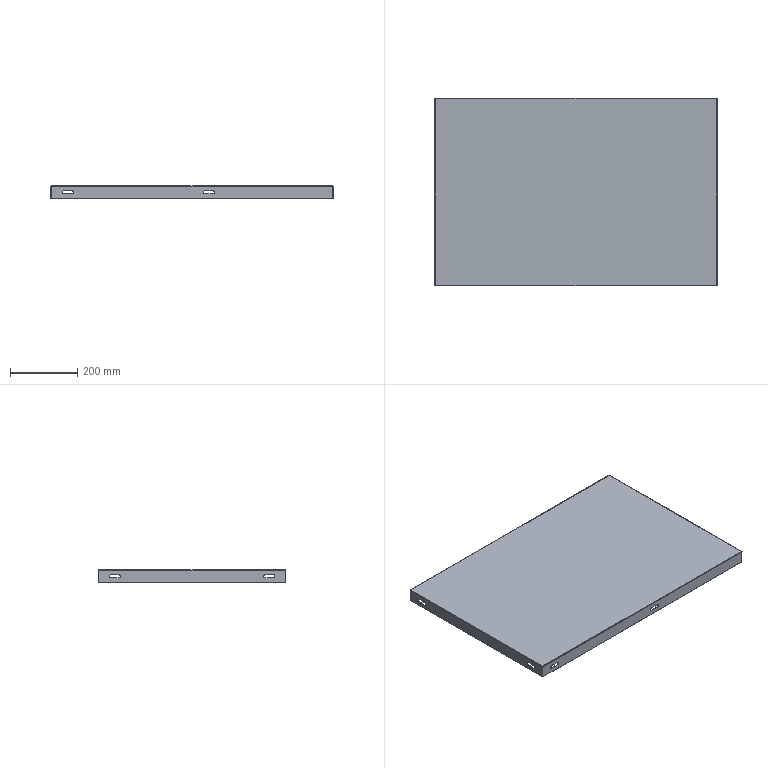Part | STEP file | Sheet-metal sealing plate_PN_0012 | 1 solid | 75 faces | box 839 x 559 x 38 mm | volume 851235 mm3 | cylinder 28 | plane 27 | spline 20 | commonest cylinder face diameters 9 x16 0.2 x4 2 x4 3.2 x4